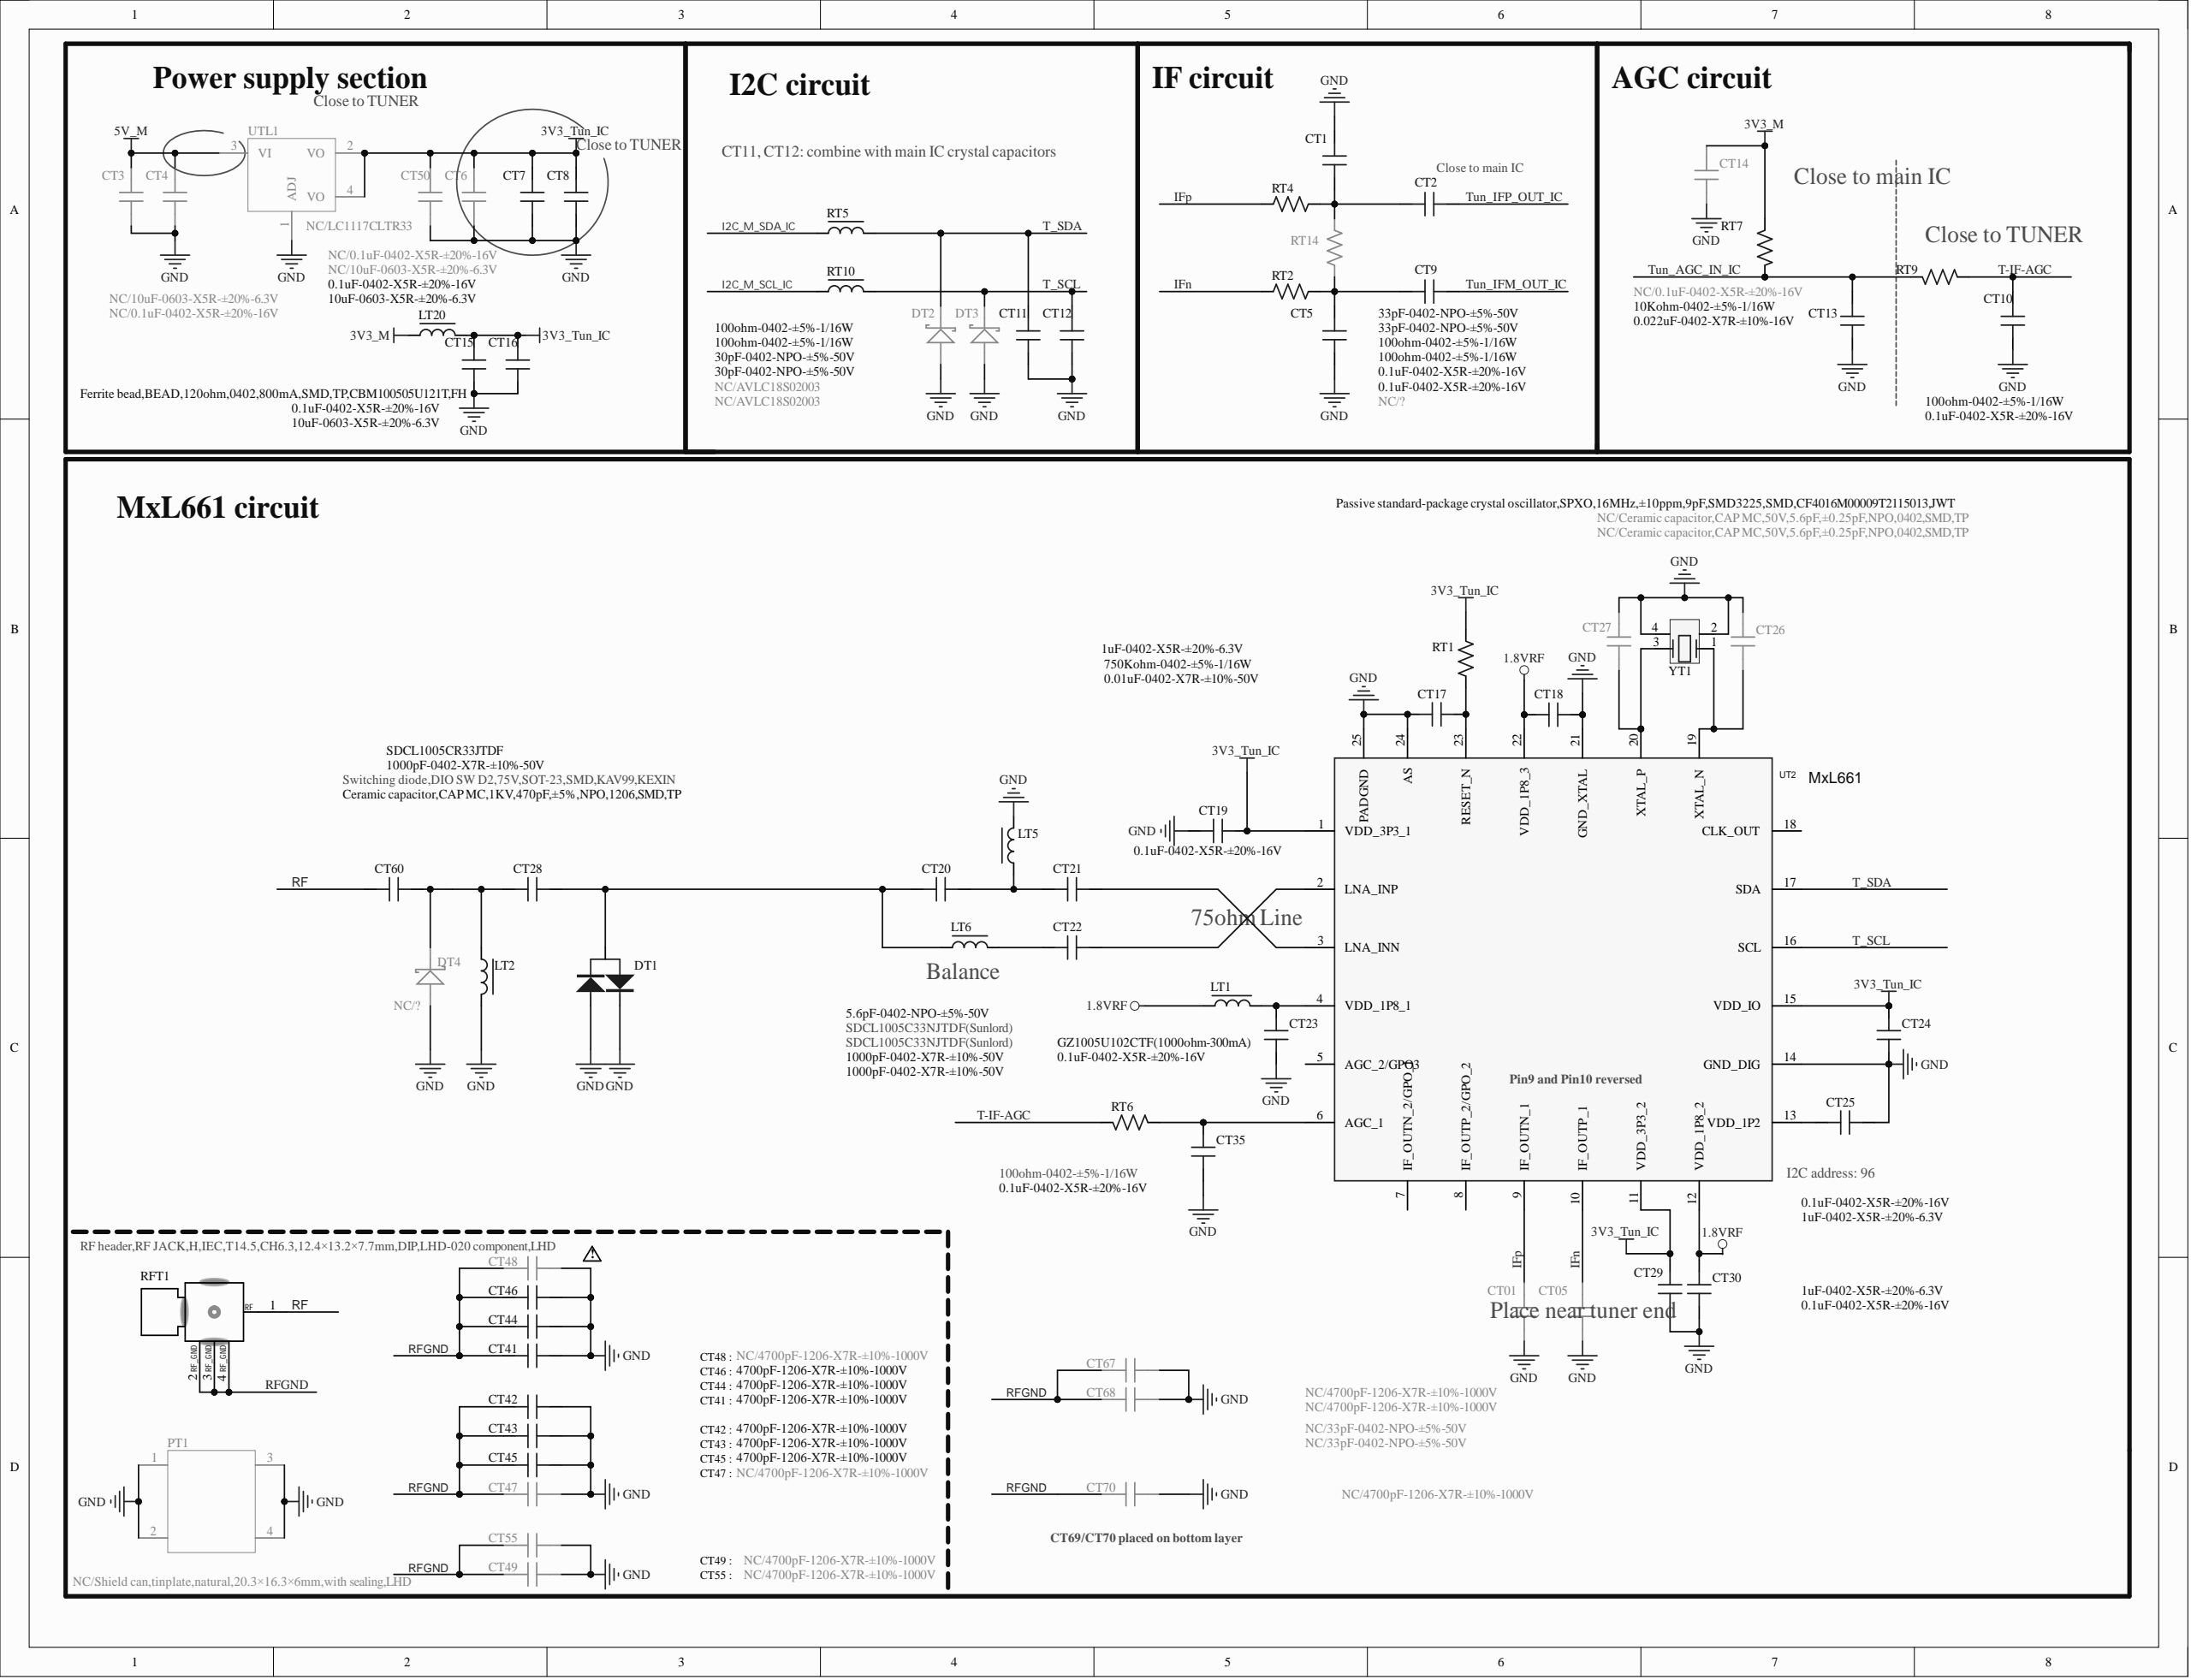Circuit board | Altium Designer | 951 parts | 509 nets | one sheet of the schematic
Parts on this sheet (reference | value | footprint):
CT1 | 33pF-0402-NPO-±5%-50V | C0402
CT01 | NC/33pF-0402-NPO-±5%-50V | C0402
CT2 | 0.1uF-0402-X5R-±20%-16V | C0402
CT3 | NC/10uF-0603-X5R-±20%-6.3V | C0603
CT4 | NC/0.1uF-0402-X5R-±20%-16V | C0402
CT5 | 33pF-0402-NPO-±5%-50V | C0402
CT05 | NC/33pF-0402-NPO-±5%-50V | C0402
CT6 | NC/0.1uF-0402-X5R-±20%-16V | C0402
CT7 | 0.1uF-0402-X5R-±20%-16V | C0402
CT8 | 10uF-0603-X5R-±20%-6.3V | C0603
CT9 | 0.1uF-0402-X5R-±20%-16V | C0402
CT10 | 0.1uF-0402-X5R-±20%-16V | C0402
CT11 | 30pF-0402-NPO-±5%-50V | C0402
CT12 | 30pF-0402-NPO-±5%-50V | C0402
CT13 | 0.022uF-0402-X7R-±10%-16V | C0402
CT14 | NC/0.1uF-0402-X5R-±20%-16V | C0402
CT15 | 10uF-0603-X5R-±20%-6.3V | C0603
CT16 | 0.1uF-0402-X5R-±20%-16V | C0402
CT17 | 1uF-0402-X5R-±20%-6.3V | C0402
CT18 | 0.01uF-0402-X7R-±10%-50V | C0402
CT19 | 0.1uF-0402-X5R-±20%-16V | C0402
CT20 | 5.6pF-0402-NPO-±5%-50V | C0402
CT21 | 1000pF-0402-X7R-±10%-50V | C0402
CT22 | 1000pF-0402-X7R-±10%-50V | C0402
CT23 | 0.1uF-0402-X5R-±20%-16V | C0402
CT24 | 0.1uF-0402-X5R-±20%-16V | C0402
CT25 | 1uF-0402-X5R-±20%-6.3V | C0402
CT26 | NC/Ceramic capacitor,CAP MC,50V,5.6pF,±0.25pF,NPO,0402,SMD,TP | C0402
CT27 | NC/Ceramic capacitor,CAP MC,50V,5.6pF,±0.25pF,NPO,0402,SMD,TP | C0402
CT28 | 1000pF-0402-X7R-±10%-50V | C0402
CT29 | 0.1uF-0402-X5R-±20%-16V | C0402
CT30 | 1uF-0402-X5R-±20%-6.3V | C0402
CT35 | 0.1uF-0402-X5R-±20%-16V | C0402
CT41 | 4700pF-1206-X7R-±10%-1000V | C1206
CT42 | 4700pF-1206-X7R-±10%-1000V | C1206
CT43 | 4700pF-1206-X7R-±10%-1000V | C1206
CT44 | 4700pF-1206-X7R-±10%-1000V | C1206
CT45 | 4700pF-1206-X7R-±10%-1000V | C1206
CT46 | 4700pF-1206-X7R-±10%-1000V | C1206
CT47 | NC/4700pF-1206-X7R-±10%-1000V | C1206
CT48 | NC/4700pF-1206-X7R-±10%-1000V | C1206
CT49 | NC/4700pF-1206-X7R-±10%-1000V | C1206
CT50 | NC/10uF-0603-X5R-±20%-6.3V | C0603
CT55 | NC/4700pF-1206-X7R-±10%-1000V | C1206
CT60 | Ceramic capacitor,CAP MC,1KV,470pF,±5%,NPO,1206,SMD,TP | C1206
CT67 | NC/4700pF-1206-X7R-±10%-1000V | C1206
CT68 | NC/4700pF-1206-X7R-±10%-1000V | C1206
CT70 | NC/4700pF-1206-X7R-±10%-1000V | C1206
DT1 | Switching diode,DIO SW D2,75V,SOT-23,SMD,KAV99,KEXIN | SO-23
DT2 | NC/AVLC18S02003 | DIODE-S0402
DT3 | NC/AVLC18S02003 | DIODE-S0402
DT4 | NC/? | DIODE-S0402
LT1 | GZ1005U102CTF(1000ohm-300mA) | L0402
LT2 | SDCL1005CR33JTDF | L0402
LT5 | SDCL1005C33NJTDF(Sunlord) | L0402
LT6 | SDCL1005C33NJTDF(Sunlord) | L0402
LT20 | Ferrite bead,BEAD,120ohm,0402,800mA,SMD,TP,CBM100505U121T,FH | L0402
PT1 | NC/Shield can,tinplate,natural,20.3×16.3×6mm,with sealing,LHD | SHIELD(16*20*6)
RFT1 | RF header,RF JACK,H,IEC,T14.5,CH6.3,12.4×13.2×7.7mm,DIP,LHD-020 component,LHD | ANT-IEC14.5-H-4
RT1 | 750Kohm-0402-±5%-1/16W | R0402
RT2 | 100ohm-0402-±5%-1/16W | R0402
RT4 | 100ohm-0402-±5%-1/16W | R0402
RT5 | 100ohm-0402-±5%-1/16W | L0402
RT6 | 100ohm-0402-±5%-1/16W | R0402
RT7 | 10Kohm-0402-±5%-1/16W | R0402
RT9 | 100ohm-0402-±5%-1/16W | R0402
RT10 | 100ohm-0402-±5%-1/16W | L0402
RT14 | NC/? | R0402
UT2 | MxL661 | QFN24/0.5-1
UTL1 | NC/LC1117CLTR33 | SOT-223
YT1 | Passive standard-package crystal oscillator,SPXO,16MHz,±10ppm,9pF,SMD3225,SMD,CF4016M00009T2115013,JWT | XTAL-S-3
Nets of these parts (net: part-pin ...):
Tun_IFP_OUT_IC: CT2-2
Tun_IFM_OUT_IC: CT9-2
Tun_AGC_IN_IC: CT13-2 RT7-2 RT9-2
T_SDA: CT11-2 DT2-K RT5-2 UT2-17
T_SCL: CT12-2 DT3-K RT10-2 UT2-16
T-IF-AGC: CT10-2 RT6-2 RT9-1
RFGND: CT41-2 CT42-2 CT43-2 CT44-2 CT45-2 CT46-2 CT47-2 CT48-2 CT49-2 CT55-2 CT67-2 CT68-2 CT70-2 RFT1-2 RFT1-3 RFT1-4
RF: CT60-1 RFT1-1
NetCT35_1: CT35-1 RT6-1 UT2-6
NetCT28_2: CT28-2 CT60-2 DT4-K LT2-1
NetCT27_2: CT27-2 YT1-3 UT2-20
NetCT26_2: CT26-2 YT1-1 UT2-19
NetCT25_2: CT25-2 UT2-13
NetCT23_1: CT23-1 LT1-2 UT2-4
NetCT22_2: CT22-2 UT2-2
NetCT22_1: CT22-1 LT6-1
NetCT21_2: CT21-2 UT2-3
NetCT20_2: CT20-2 CT21-1 LT5-2
NetCT20_1: CT20-1 CT28-1 DT1-2 LT6-2
NetCT17_2: CT17-2 RT1-1 UT2-23
NetCT5_2: CT5-2 CT9-1 RT2-2 RT14-1
NetCT1_1: CT1-1 CT2-1 RT4-2 RT14-2
IFp: CT01-2 RT4-1 UT2-9
IFn: CT05-2 RT2-1 UT2-10
I2C_M_SDA_IC: RT5-1
I2C_M_SCL_IC: RT10-1
GND: CT01-1 CT1-2 CT3-1 CT4-2 CT5-1 CT05-1 CT6-1 CT7-1 CT8-2 CT10-1 CT11-1 CT12-1 CT13-1 CT14-2 CT15-1 CT16-1 CT17-1 CT18-2 CT19-2 CT23-2 CT24-2 CT25-1 CT26-1 CT27-1 CT29-1 CT30-1 CT35-2 CT41-1 CT42-1 CT43-1 CT44-1 CT45-1 CT46-1 CT47-1 CT48-1 CT49-1 CT50-1 CT55-1 CT67-1 CT68-1 CT70-1 DT1-1 DT1-3 DT2-A DT3-A DT4-A LT2-2 LT5-1 PT1-1 PT1-2 PT1-3 PT1-4 UTL1-1 YT1-2 YT1-4 UT2-14 UT2-21 UT2-24 UT2-25
5V_M: CT3-2 CT4-1 UTL1-3
3V3_Tun_IC: CT6-2 CT7-2 CT8-1 CT15-2 CT16-2 CT19-1 CT24-1 CT29-2 CT50-2 LT20-2 RT1-2 UTL1-2 UTL1-4 UT2-1 UT2-11 UT2-15
3V3_M: CT14-1 LT20-1 RT7-1
1.8VRF: CT18-1 CT30-2 LT1-1 UT2-12 UT2-22